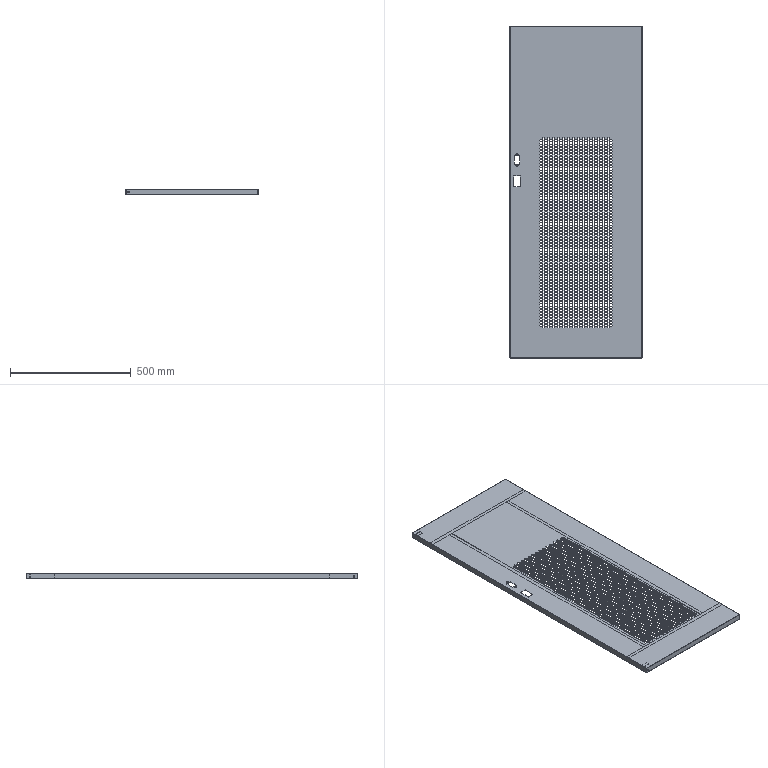Part | SolidWorks | features MirrorCompFeat 1, ReferencePattern 1 | 7 solids | 11628 faces | volume 1001235 mm3 | plane 11528 | cylinder 84 | spline 16 | commonest cylinder face diameters 4.5 x16 0.2 x14 5.5 x12 6.5 x12 11.5 x12 2.6 x8